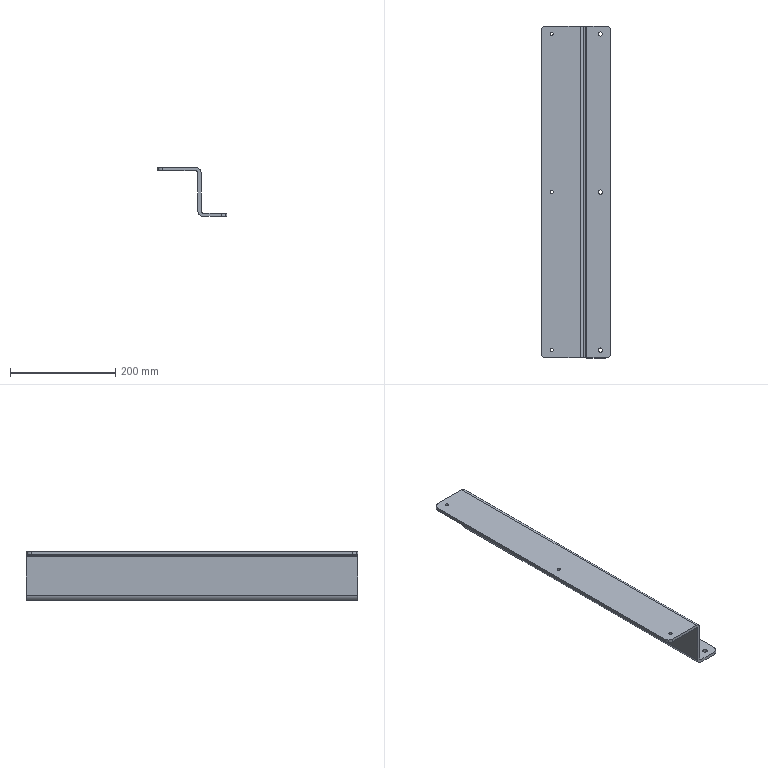Part | STEP file | SUPPORT.BRACKET.21.stp | 1 solid | 38 faces | box 132.5 x 630 x 92 mm | volume 804533 mm3 | cylinder 28 | plane 6 | spline 4 | commonest cylinder face diameters 6 x10 20 x8 8 x6 18 x4